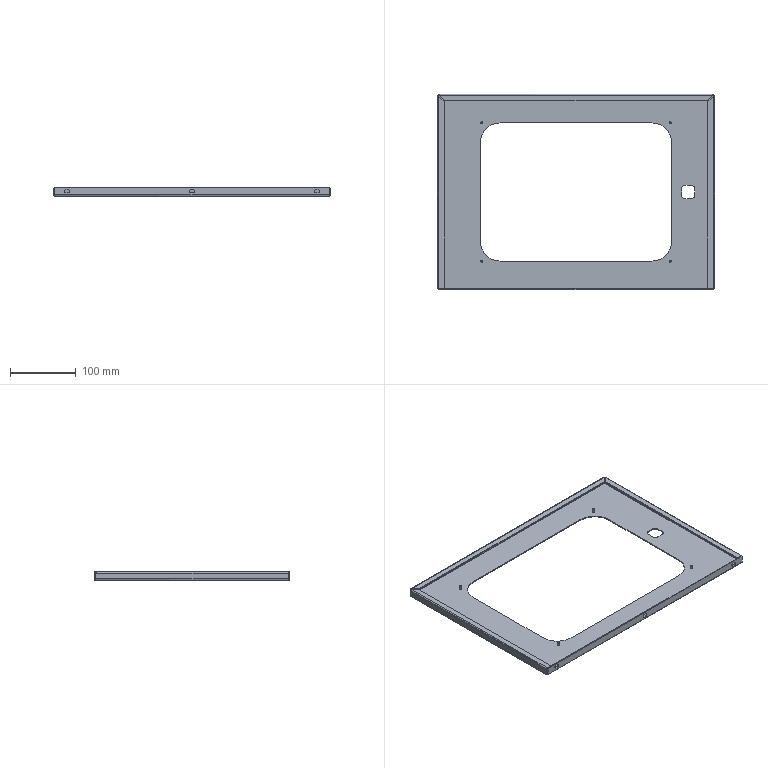Part | SolidWorks | features BaseBody 1 | 1 solid | 102 faces | box 421 x 297 x 13 mm | volume 131507 mm3 | plane 54 | cylinder 36 | spline 12 | commonest cylinder face diameters 3 x8 1 x7 4 x7 5 x6 10 x4 60 x4